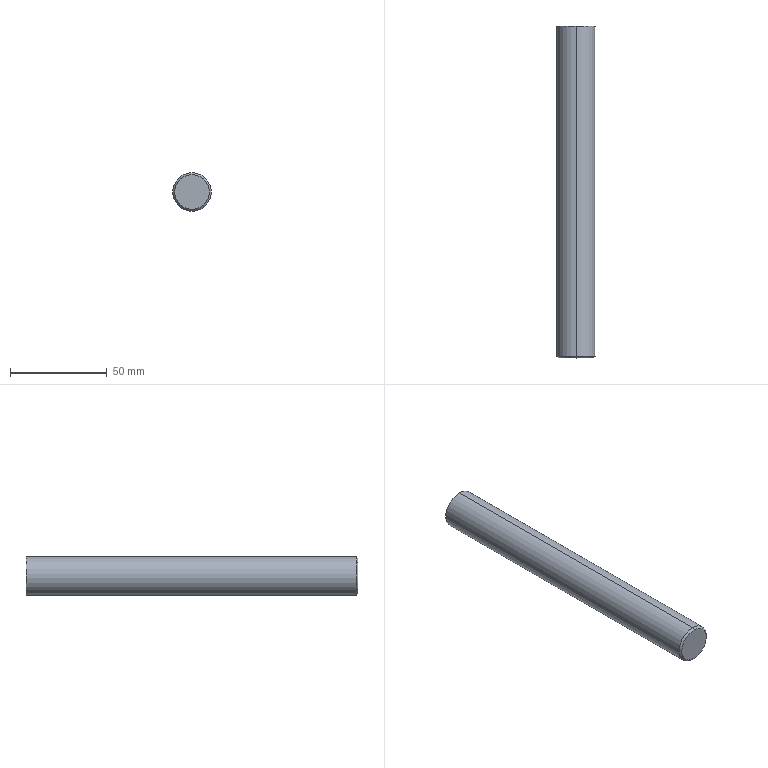Part | SolidWorks | features Chamfer 1, Extrusion 1 | 1 solid | 6 faces | box 20 x 172 x 20 mm | volume 54005 mm3 | cone 2 | cylinder 2 | plane 2 | commonest cylinder face diameters 20 x2
STEP:
#1=CARTESIAN_POINT('',(0.,0.,-9.));
#2=VERTEX_POINT('',#1);
#3=CARTESIAN_POINT('',(0.,0.,9.));
#4=VERTEX_POINT('',#3);
#5=CARTESIAN_POINT('',(0.,0.,0.));
#6=DIRECTION('',(0.,-1.,0.));
#7=DIRECTION('',(0.,0.,1.));
#8=AXIS2_PLACEMENT_3D('',#5,#6,#7);
#9=CIRCLE('',#8,9.);
#10=EDGE_CURVE('',#2,#4,#9,.T.);
#11=ORIENTED_EDGE('',*,*,#10,.F.);
#12=CARTESIAN_POINT('',(0.,1.,-10.));
#13=VERTEX_POINT('',#12);
#14=CARTESIAN_POINT('',(0.,1.,-10.));
#15=DIRECTION('',(0.,0.7071,-0.7071));
#16=VECTOR('',#15,1000.);
#17=LINE('',#14,#16);
#18=EDGE_CURVE('',#2,#13,#17,.T.);
#19=ORIENTED_EDGE('',*,*,#18,.T.);
#20=CARTESIAN_POINT('',(0.,1.,10.));
#21=VERTEX_POINT('',#20);
#22=CARTESIAN_POINT('',(0.,1.,0.));
#23=DIRECTION('',(0.,1.,0.));
#24=DIRECTION('',(0.,0.,1.));
#25=AXIS2_PLACEMENT_3D('',#22,#23,#24);
#26=CIRCLE('',#25,10.);
#27=EDGE_CURVE('',#21,#13,#26,.T.);
#28=ORIENTED_EDGE('',*,*,#27,.F.);
#29=CARTESIAN_POINT('',(0.,1.,10.));
#30=DIRECTION('',(0.,0.7071,0.7071));
#31=VECTOR('',#30,1000.);
#32=LINE('',#29,#31);
#33=EDGE_CURVE('',#4,#21,#32,.T.);
#34=ORIENTED_EDGE('',*,*,#33,.F.);
#35=EDGE_LOOP('',(#11,#19,#28,#34));
#36=FACE_OUTER_BOUND('',#35,.T.);
#37=CARTESIAN_POINT('',(0.,1.,0.));
#38=DIRECTION('',(0.,1.,0.));
#39=DIRECTION('',(0.,0.,1.));
#40=AXIS2_PLACEMENT_3D('',#37,#38,#39);
#41=CONICAL_SURFACE('',#40,10.,0.7854);
#42=ADVANCED_FACE('',(#36),#41,.T.);
#43=CARTESIAN_POINT('',(0.,172.,10.));
#44=VERTEX_POINT('',#43);
#45=CARTESIAN_POINT('',(0.,172.,-10.));
#46=VERTEX_POINT('',#45);
#47=CARTESIAN_POINT('',(0.,172.,0.));
#48=DIRECTION('',(0.,1.,0.));
#49=DIRECTION('',(0.,0.,1.));
#50=AXIS2_PLACEMENT_3D('',#47,#48,#49);
#51=CIRCLE('',#50,10.);
#52=EDGE_CURVE('',#44,#46,#51,.T.);
#53=ORIENTED_EDGE('',*,*,#52,.F.);
#54=CARTESIAN_POINT('',(0.,172.,10.));
#55=DIRECTION('',(0.,-1.,0.));
#56=VECTOR('',#55,1000.);
#57=LINE('',#54,#56);
#58=EDGE_CURVE('',#44,#21,#57,.T.);
#59=ORIENTED_EDGE('',*,*,#58,.T.);
#60=ORIENTED_EDGE('',*,*,#27,.T.);
#61=CARTESIAN_POINT('',(0.,172.,-10.));
#62=DIRECTION('',(0.,-1.,0.));
#63=VECTOR('',#62,1000.);
#64=LINE('',#61,#63);
#65=EDGE_CURVE('',#46,#13,#64,.T.);
#66=ORIENTED_EDGE('',*,*,#65,.F.);
#67=EDGE_LOOP('',(#53,#59,#60,#66));
#68=FACE_OUTER_BOUND('',#67,.T.);
#69=CARTESIAN_POINT('',(0.,172.,0.));
#70=DIRECTION('',(0.,-1.,0.));
#71=DIRECTION('',(0.,0.,-1.));
#72=AXIS2_PLACEMENT_3D('',#69,#70,#71);
#73=CYLINDRICAL_SURFACE('',#72,10.);
#74=ADVANCED_FACE('',(#68),#73,.T.);
#75=ORIENTED_EDGE('',*,*,#58,.F.);
#76=CARTESIAN_POINT('',(0.,172.,0.));
#77=DIRECTION('',(0.,1.,0.));
#78=DIRECTION('',(0.,0.,1.));
#79=AXIS2_PLACEMENT_3D('',#76,#77,#78);
#80=CIRCLE('',#79,10.);
#81=EDGE_CURVE('',#46,#44,#80,.T.);
#82=ORIENTED_EDGE('',*,*,#81,.F.);
#83=ORIENTED_EDGE('',*,*,#65,.T.);
#84=CARTESIAN_POINT('',(0.,1.,0.));
#85=DIRECTION('',(0.,1.,0.));
#86=DIRECTION('',(0.,0.,1.));
#87=AXIS2_PLACEMENT_3D('',#84,#85,#86);
#88=CIRCLE('',#87,10.);
#89=EDGE_CURVE('',#13,#21,#88,.T.);
#90=ORIENTED_EDGE('',*,*,#89,.T.);
#91=EDGE_LOOP('',(#75,#82,#83,#90));
#92=FACE_OUTER_BOUND('',#91,.T.);
#93=CARTESIAN_POINT('',(0.,172.,0.));
#94=DIRECTION('',(0.,-1.,0.));
#95=DIRECTION('',(0.,0.,-1.));
#96=AXIS2_PLACEMENT_3D('',#93,#94,#95);
#97=CYLINDRICAL_SURFACE('',#96,10.);
#98=ADVANCED_FACE('',(#92),#97,.T.);
#99=ORIENTED_EDGE('',*,*,#81,.T.);
#100=ORIENTED_EDGE('',*,*,#52,.T.);
#101=EDGE_LOOP('',(#99,#100));
#102=FACE_OUTER_BOUND('',#101,.T.);
#103=CARTESIAN_POINT('',(0.,172.,0.));
#104=DIRECTION('',(0.,1.,0.));
#105=DIRECTION('',(0.,0.,1.));
#106=AXIS2_PLACEMENT_3D('',#103,#104,#105);
#107=PLANE('',#106);
#108=ADVANCED_FACE('',(#102),#107,.T.);
#109=CARTESIAN_POINT('',(0.,0.,0.));
#110=DIRECTION('',(0.,-1.,0.));
#111=DIRECTION('',(0.,0.,1.));
#112=AXIS2_PLACEMENT_3D('',#109,#110,#111);
#113=CIRCLE('',#112,9.);
#114=EDGE_CURVE('',#4,#2,#113,.T.);
#115=ORIENTED_EDGE('',*,*,#114,.T.);
#116=ORIENTED_EDGE('',*,*,#10,.T.);
#117=EDGE_LOOP('',(#115,#116));
#118=FACE_OUTER_BOUND('',#117,.T.);
#119=CARTESIAN_POINT('',(0.,0.,0.));
#120=DIRECTION('',(0.,1.,0.));
#121=DIRECTION('',(0.,0.,1.));
#122=AXIS2_PLACEMENT_3D('',#119,#120,#121);
#123=PLANE('',#122);
#124=ADVANCED_FACE('',(#118),#123,.F.);
#125=ORIENTED_EDGE('',*,*,#18,.F.);
#126=ORIENTED_EDGE('',*,*,#114,.F.);
#127=ORIENTED_EDGE('',*,*,#33,.T.);
#128=ORIENTED_EDGE('',*,*,#89,.F.);
#129=EDGE_LOOP('',(#125,#126,#127,#128));
#130=FACE_OUTER_BOUND('',#129,.T.);
#131=CARTESIAN_POINT('',(0.,1.,0.));
#132=DIRECTION('',(0.,1.,0.));
#133=DIRECTION('',(0.,0.,1.));
#134=AXIS2_PLACEMENT_3D('',#131,#132,#133);
#135=CONICAL_SURFACE('',#134,10.,0.7854);
#136=ADVANCED_FACE('',(#130),#135,.T.);
#137=CLOSED_SHELL('',(#42,#74,#98,#108,#124,#136));
#138=MANIFOLD_SOLID_BREP('',#137);
#139=CARTESIAN_POINT('',(0.,0.,0.));
#140=DIRECTION('',(0.,0.,1.));
#141=DIRECTION('',(1.,0.,0.));
#142=AXIS2_PLACEMENT_3D('',#139,#140,#141);
#143=(LENGTH_UNIT()NAMED_UNIT(*)SI_UNIT(.MILLI.,.METRE.));
#144=UNCERTAINTY_MEASURE_WITH_UNIT(LENGTH_MEASURE(0.00001),#143,'','');
#145=(NAMED_UNIT(*)PLANE_ANGLE_UNIT()SI_UNIT($,.RADIAN.));
#146=(NAMED_UNIT(*)SI_UNIT($,.STERADIAN.)SOLID_ANGLE_UNIT());
#147=(GEOMETRIC_REPRESENTATION_CONTEXT(3)GLOBAL_UNCERTAINTY_ASSIGNED_CONTEXT((#144))GLOBAL_UNIT_ASSIGNED_CONTEXT((#143,#145,#146))REPRESENTATION_CONTEXT('',''));
#148=ADVANCED_BREP_SHAPE_REPRESENTATION('',(#138,#142),#147);